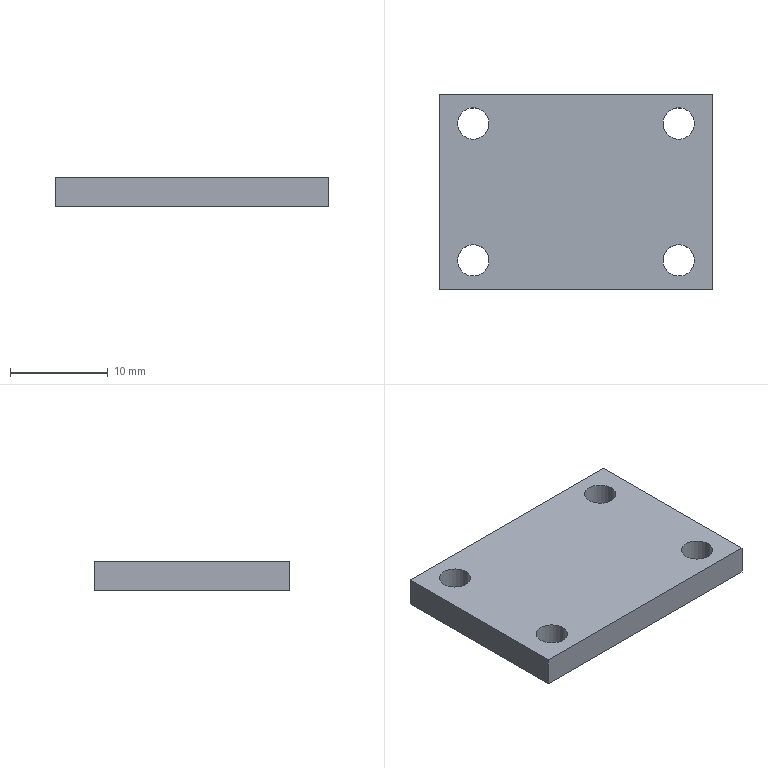Part | SolidWorks | features Extrusion 1 | 1 solid | 14 faces | box 28 x 20 x 3 mm | volume 1583 mm3 | cylinder 8 | plane 6 | commonest cylinder face diameters 3.2 x8
STEP:
#1=CARTESIAN_POINT('',(-12.1,-7.,1.5));
#2=VERTEX_POINT('',#1);
#3=CARTESIAN_POINT('',(-8.9,-7.,1.5));
#4=VERTEX_POINT('',#3);
#5=CARTESIAN_POINT('',(-10.5,-7.,1.5));
#6=DIRECTION('',(0.,0.,1.));
#7=DIRECTION('',(1.,0.,0.));
#8=AXIS2_PLACEMENT_3D('',#5,#6,#7);
#9=CIRCLE('',#8,1.6);
#10=EDGE_CURVE('',#2,#4,#9,.T.);
#11=ORIENTED_EDGE('',*,*,#10,.T.);
#12=CARTESIAN_POINT('',(-8.9,-7.,-1.5));
#13=VERTEX_POINT('',#12);
#14=CARTESIAN_POINT('',(-8.9,-7.,1.5));
#15=DIRECTION('',(0.,0.,-1.));
#16=VECTOR('',#15,1000.);
#17=LINE('',#14,#16);
#18=EDGE_CURVE('',#4,#13,#17,.T.);
#19=ORIENTED_EDGE('',*,*,#18,.T.);
#20=CARTESIAN_POINT('',(-12.1,-7.,-1.5));
#21=VERTEX_POINT('',#20);
#22=CARTESIAN_POINT('',(-10.5,-7.,-1.5));
#23=DIRECTION('',(0.,0.,1.));
#24=DIRECTION('',(1.,0.,0.));
#25=AXIS2_PLACEMENT_3D('',#22,#23,#24);
#26=CIRCLE('',#25,1.6);
#27=EDGE_CURVE('',#21,#13,#26,.T.);
#28=ORIENTED_EDGE('',*,*,#27,.F.);
#29=CARTESIAN_POINT('',(-12.1,-7.,1.5));
#30=DIRECTION('',(0.,0.,-1.));
#31=VECTOR('',#30,1000.);
#32=LINE('',#29,#31);
#33=EDGE_CURVE('',#2,#21,#32,.T.);
#34=ORIENTED_EDGE('',*,*,#33,.F.);
#35=EDGE_LOOP('',(#11,#19,#28,#34));
#36=FACE_OUTER_BOUND('',#35,.T.);
#37=CARTESIAN_POINT('',(-10.5,-7.,1.5));
#38=DIRECTION('',(0.,0.,-1.));
#39=DIRECTION('',(-1.,0.,0.));
#40=AXIS2_PLACEMENT_3D('',#37,#38,#39);
#41=CYLINDRICAL_SURFACE('',#40,1.6);
#42=ADVANCED_FACE('',(#36),#41,.F.);
#43=CARTESIAN_POINT('',(8.9,-7.,1.5));
#44=VERTEX_POINT('',#43);
#45=CARTESIAN_POINT('',(12.1,-7.,1.5));
#46=VERTEX_POINT('',#45);
#47=CARTESIAN_POINT('',(10.5,-7.,1.5));
#48=DIRECTION('',(0.,0.,1.));
#49=DIRECTION('',(-1.,0.,0.));
#50=AXIS2_PLACEMENT_3D('',#47,#48,#49);
#51=CIRCLE('',#50,1.6);
#52=EDGE_CURVE('',#44,#46,#51,.T.);
#53=ORIENTED_EDGE('',*,*,#52,.T.);
#54=CARTESIAN_POINT('',(12.1,-7.,-1.5));
#55=VERTEX_POINT('',#54);
#56=CARTESIAN_POINT('',(12.1,-7.,1.5));
#57=DIRECTION('',(0.,0.,-1.));
#58=VECTOR('',#57,1000.);
#59=LINE('',#56,#58);
#60=EDGE_CURVE('',#46,#55,#59,.T.);
#61=ORIENTED_EDGE('',*,*,#60,.T.);
#62=CARTESIAN_POINT('',(8.9,-7.,-1.5));
#63=VERTEX_POINT('',#62);
#64=CARTESIAN_POINT('',(10.5,-7.,-1.5));
#65=DIRECTION('',(0.,0.,1.));
#66=DIRECTION('',(-1.,0.,0.));
#67=AXIS2_PLACEMENT_3D('',#64,#65,#66);
#68=CIRCLE('',#67,1.6);
#69=EDGE_CURVE('',#63,#55,#68,.T.);
#70=ORIENTED_EDGE('',*,*,#69,.F.);
#71=CARTESIAN_POINT('',(8.9,-7.,1.5));
#72=DIRECTION('',(0.,0.,-1.));
#73=VECTOR('',#72,1000.);
#74=LINE('',#71,#73);
#75=EDGE_CURVE('',#44,#63,#74,.T.);
#76=ORIENTED_EDGE('',*,*,#75,.F.);
#77=EDGE_LOOP('',(#53,#61,#70,#76));
#78=FACE_OUTER_BOUND('',#77,.T.);
#79=CARTESIAN_POINT('',(10.5,-7.,1.5));
#80=DIRECTION('',(0.,0.,-1.));
#81=DIRECTION('',(-1.,0.,0.));
#82=AXIS2_PLACEMENT_3D('',#79,#80,#81);
#83=CYLINDRICAL_SURFACE('',#82,1.6);
#84=ADVANCED_FACE('',(#78),#83,.F.);
#85=CARTESIAN_POINT('',(-12.1,7.,1.5));
#86=VERTEX_POINT('',#85);
#87=CARTESIAN_POINT('',(-8.9,7.,1.5));
#88=VERTEX_POINT('',#87);
#89=CARTESIAN_POINT('',(-10.5,7.,1.5));
#90=DIRECTION('',(0.,0.,1.));
#91=DIRECTION('',(-1.,0.,0.));
#92=AXIS2_PLACEMENT_3D('',#89,#90,#91);
#93=CIRCLE('',#92,1.6);
#94=EDGE_CURVE('',#86,#88,#93,.T.);
#95=ORIENTED_EDGE('',*,*,#94,.T.);
#96=CARTESIAN_POINT('',(-8.9,7.,-1.5));
#97=VERTEX_POINT('',#96);
#98=CARTESIAN_POINT('',(-8.9,7.,1.5));
#99=DIRECTION('',(0.,0.,-1.));
#100=VECTOR('',#99,1000.);
#101=LINE('',#98,#100);
#102=EDGE_CURVE('',#88,#97,#101,.T.);
#103=ORIENTED_EDGE('',*,*,#102,.T.);
#104=CARTESIAN_POINT('',(-12.1,7.,-1.5));
#105=VERTEX_POINT('',#104);
#106=CARTESIAN_POINT('',(-10.5,7.,-1.5));
#107=DIRECTION('',(0.,0.,1.));
#108=DIRECTION('',(-1.,0.,0.));
#109=AXIS2_PLACEMENT_3D('',#106,#107,#108);
#110=CIRCLE('',#109,1.6);
#111=EDGE_CURVE('',#105,#97,#110,.T.);
#112=ORIENTED_EDGE('',*,*,#111,.F.);
#113=CARTESIAN_POINT('',(-12.1,7.,1.5));
#114=DIRECTION('',(0.,0.,-1.));
#115=VECTOR('',#114,1000.);
#116=LINE('',#113,#115);
#117=EDGE_CURVE('',#86,#105,#116,.T.);
#118=ORIENTED_EDGE('',*,*,#117,.F.);
#119=EDGE_LOOP('',(#95,#103,#112,#118));
#120=FACE_OUTER_BOUND('',#119,.T.);
#121=CARTESIAN_POINT('',(-10.5,7.,1.5));
#122=DIRECTION('',(0.,0.,-1.));
#123=DIRECTION('',(-1.,0.,0.));
#124=AXIS2_PLACEMENT_3D('',#121,#122,#123);
#125=CYLINDRICAL_SURFACE('',#124,1.6);
#126=ADVANCED_FACE('',(#120),#125,.F.);
#127=CARTESIAN_POINT('',(8.9,7.,1.5));
#128=VERTEX_POINT('',#127);
#129=CARTESIAN_POINT('',(12.1,7.,1.5));
#130=VERTEX_POINT('',#129);
#131=CARTESIAN_POINT('',(10.5,7.,1.5));
#132=DIRECTION('',(0.,0.,1.));
#133=DIRECTION('',(1.,0.,0.));
#134=AXIS2_PLACEMENT_3D('',#131,#132,#133);
#135=CIRCLE('',#134,1.6);
#136=EDGE_CURVE('',#128,#130,#135,.T.);
#137=ORIENTED_EDGE('',*,*,#136,.T.);
#138=CARTESIAN_POINT('',(12.1,7.,-1.5));
#139=VERTEX_POINT('',#138);
#140=CARTESIAN_POINT('',(12.1,7.,1.5));
#141=DIRECTION('',(0.,0.,-1.));
#142=VECTOR('',#141,1000.);
#143=LINE('',#140,#142);
#144=EDGE_CURVE('',#130,#139,#143,.T.);
#145=ORIENTED_EDGE('',*,*,#144,.T.);
#146=CARTESIAN_POINT('',(8.9,7.,-1.5));
#147=VERTEX_POINT('',#146);
#148=CARTESIAN_POINT('',(10.5,7.,-1.5));
#149=DIRECTION('',(0.,0.,1.));
#150=DIRECTION('',(1.,0.,0.));
#151=AXIS2_PLACEMENT_3D('',#148,#149,#150);
#152=CIRCLE('',#151,1.6);
#153=EDGE_CURVE('',#147,#139,#152,.T.);
#154=ORIENTED_EDGE('',*,*,#153,.F.);
#155=CARTESIAN_POINT('',(8.9,7.,1.5));
#156=DIRECTION('',(0.,0.,-1.));
#157=VECTOR('',#156,1000.);
#158=LINE('',#155,#157);
#159=EDGE_CURVE('',#128,#147,#158,.T.);
#160=ORIENTED_EDGE('',*,*,#159,.F.);
#161=EDGE_LOOP('',(#137,#145,#154,#160));
#162=FACE_OUTER_BOUND('',#161,.T.);
#163=CARTESIAN_POINT('',(10.5,7.,1.5));
#164=DIRECTION('',(0.,0.,-1.));
#165=DIRECTION('',(-1.,0.,0.));
#166=AXIS2_PLACEMENT_3D('',#163,#164,#165);
#167=CYLINDRICAL_SURFACE('',#166,1.6);
#168=ADVANCED_FACE('',(#162),#167,.F.);
#169=CARTESIAN_POINT('',(-14.,10.,1.5));
#170=VERTEX_POINT('',#169);
#171=CARTESIAN_POINT('',(-14.,-10.,1.5));
#172=VERTEX_POINT('',#171);
#173=CARTESIAN_POINT('',(-14.,10.,1.5));
#174=DIRECTION('',(0.,-1.,0.));
#175=VECTOR('',#174,1000.);
#176=LINE('',#173,#175);
#177=EDGE_CURVE('',#170,#172,#176,.T.);
#178=ORIENTED_EDGE('',*,*,#177,.T.);
#179=CARTESIAN_POINT('',(14.,-10.,1.5));
#180=VERTEX_POINT('',#179);
#181=CARTESIAN_POINT('',(14.,-10.,1.5));
#182=DIRECTION('',(1.,0.,0.));
#183=VECTOR('',#182,1000.);
#184=LINE('',#181,#183);
#185=EDGE_CURVE('',#172,#180,#184,.T.);
#186=ORIENTED_EDGE('',*,*,#185,.T.);
#187=CARTESIAN_POINT('',(14.,10.,1.5));
#188=VERTEX_POINT('',#187);
#189=CARTESIAN_POINT('',(14.,10.,1.5));
#190=DIRECTION('',(0.,1.,0.));
#191=VECTOR('',#190,1000.);
#192=LINE('',#189,#191);
#193=EDGE_CURVE('',#180,#188,#192,.T.);
#194=ORIENTED_EDGE('',*,*,#193,.T.);
#195=CARTESIAN_POINT('',(14.,10.,1.5));
#196=DIRECTION('',(-1.,0.,0.));
#197=VECTOR('',#196,1000.);
#198=LINE('',#195,#197);
#199=EDGE_CURVE('',#188,#170,#198,.T.);
#200=ORIENTED_EDGE('',*,*,#199,.T.);
#201=EDGE_LOOP('',(#178,#186,#194,#200));
#202=FACE_OUTER_BOUND('',#201,.T.);
#203=ORIENTED_EDGE('',*,*,#136,.F.);
#204=CARTESIAN_POINT('',(10.5,7.,1.5));
#205=DIRECTION('',(0.,0.,1.));
#206=DIRECTION('',(1.,0.,0.));
#207=AXIS2_PLACEMENT_3D('',#204,#205,#206);
#208=CIRCLE('',#207,1.6);
#209=EDGE_CURVE('',#130,#128,#208,.T.);
#210=ORIENTED_EDGE('',*,*,#209,.F.);
#211=EDGE_LOOP('',(#203,#210));
#212=FACE_BOUND('',#211,.T.);
#213=ORIENTED_EDGE('',*,*,#94,.F.);
#214=CARTESIAN_POINT('',(-10.5,7.,1.5));
#215=DIRECTION('',(0.,0.,1.));
#216=DIRECTION('',(-1.,0.,0.));
#217=AXIS2_PLACEMENT_3D('',#214,#215,#216);
#218=CIRCLE('',#217,1.6);
#219=EDGE_CURVE('',#88,#86,#218,.T.);
#220=ORIENTED_EDGE('',*,*,#219,.F.);
#221=EDGE_LOOP('',(#213,#220));
#222=FACE_BOUND('',#221,.T.);
#223=ORIENTED_EDGE('',*,*,#52,.F.);
#224=CARTESIAN_POINT('',(10.5,-7.,1.5));
#225=DIRECTION('',(0.,0.,1.));
#226=DIRECTION('',(-1.,0.,0.));
#227=AXIS2_PLACEMENT_3D('',#224,#225,#226);
#228=CIRCLE('',#227,1.6);
#229=EDGE_CURVE('',#46,#44,#228,.T.);
#230=ORIENTED_EDGE('',*,*,#229,.F.);
#231=EDGE_LOOP('',(#223,#230));
#232=FACE_BOUND('',#231,.T.);
#233=ORIENTED_EDGE('',*,*,#10,.F.);
#234=CARTESIAN_POINT('',(-10.5,-7.,1.5));
#235=DIRECTION('',(0.,0.,1.));
#236=DIRECTION('',(1.,0.,0.));
#237=AXIS2_PLACEMENT_3D('',#234,#235,#236);
#238=CIRCLE('',#237,1.6);
#239=EDGE_CURVE('',#4,#2,#238,.T.);
#240=ORIENTED_EDGE('',*,*,#239,.F.);
#241=EDGE_LOOP('',(#233,#240));
#242=FACE_BOUND('',#241,.T.);
#243=CARTESIAN_POINT('',(0.,0.,1.5));
#244=DIRECTION('',(0.,0.,-1.));
#245=DIRECTION('',(-1.,0.,0.));
#246=AXIS2_PLACEMENT_3D('',#243,#244,#245);
#247=PLANE('',#246);
#248=ADVANCED_FACE('',(#202,#212,#222,#232,#242),#247,.F.);
#249=ORIENTED_EDGE('',*,*,#69,.T.);
#250=CARTESIAN_POINT('',(10.5,-7.,-1.5));
#251=DIRECTION('',(0.,0.,1.));
#252=DIRECTION('',(-1.,0.,0.));
#253=AXIS2_PLACEMENT_3D('',#250,#251,#252);
#254=CIRCLE('',#253,1.6);
#255=EDGE_CURVE('',#55,#63,#254,.T.);
#256=ORIENTED_EDGE('',*,*,#255,.T.);
#257=EDGE_LOOP('',(#249,#256));
#258=FACE_BOUND('',#257,.T.);
#259=ORIENTED_EDGE('',*,*,#153,.T.);
#260=CARTESIAN_POINT('',(10.5,7.,-1.5));
#261=DIRECTION('',(0.,0.,1.));
#262=DIRECTION('',(1.,0.,0.));
#263=AXIS2_PLACEMENT_3D('',#260,#261,#262);
#264=CIRCLE('',#263,1.6);
#265=EDGE_CURVE('',#139,#147,#264,.T.);
#266=ORIENTED_EDGE('',*,*,#265,.T.);
#267=EDGE_LOOP('',(#259,#266));
#268=FACE_BOUND('',#267,.T.);
#269=CARTESIAN_POINT('',(-14.,10.,-1.5));
#270=VERTEX_POINT('',#269);
#271=CARTESIAN_POINT('',(-14.,-10.,-1.5));
#272=VERTEX_POINT('',#271);
#273=CARTESIAN_POINT('',(-14.,10.,-1.5));
#274=DIRECTION('',(0.,-1.,0.));
#275=VECTOR('',#274,1000.);
#276=LINE('',#273,#275);
#277=EDGE_CURVE('',#270,#272,#276,.T.);
#278=ORIENTED_EDGE('',*,*,#277,.F.);
#279=CARTESIAN_POINT('',(14.,10.,-1.5));
#280=VERTEX_POINT('',#279);
#281=CARTESIAN_POINT('',(14.,10.,-1.5));
#282=DIRECTION('',(-1.,0.,0.));
#283=VECTOR('',#282,1000.);
#284=LINE('',#281,#283);
#285=EDGE_CURVE('',#280,#270,#284,.T.);
#286=ORIENTED_EDGE('',*,*,#285,.F.);
#287=CARTESIAN_POINT('',(14.,-10.,-1.5));
#288=VERTEX_POINT('',#287);
#289=CARTESIAN_POINT('',(14.,10.,-1.5));
#290=DIRECTION('',(0.,1.,0.));
#291=VECTOR('',#290,1000.);
#292=LINE('',#289,#291);
#293=EDGE_CURVE('',#288,#280,#292,.T.);
#294=ORIENTED_EDGE('',*,*,#293,.F.);
#295=CARTESIAN_POINT('',(14.,-10.,-1.5));
#296=DIRECTION('',(1.,0.,0.));
#297=VECTOR('',#296,1000.);
#298=LINE('',#295,#297);
#299=EDGE_CURVE('',#272,#288,#298,.T.);
#300=ORIENTED_EDGE('',*,*,#299,.F.);
#301=EDGE_LOOP('',(#278,#286,#294,#300));
#302=FACE_OUTER_BOUND('',#301,.T.);
#303=ORIENTED_EDGE('',*,*,#111,.T.);
#304=CARTESIAN_POINT('',(-10.5,7.,-1.5));
#305=DIRECTION('',(0.,0.,1.));
#306=DIRECTION('',(-1.,0.,0.));
#307=AXIS2_PLACEMENT_3D('',#304,#305,#306);
#308=CIRCLE('',#307,1.6);
#309=EDGE_CURVE('',#97,#105,#308,.T.);
#310=ORIENTED_EDGE('',*,*,#309,.T.);
#311=EDGE_LOOP('',(#303,#310));
#312=FACE_BOUND('',#311,.T.);
#313=ORIENTED_EDGE('',*,*,#27,.T.);
#314=CARTESIAN_POINT('',(-10.5,-7.,-1.5));
#315=DIRECTION('',(0.,0.,1.));
#316=DIRECTION('',(1.,0.,0.));
#317=AXIS2_PLACEMENT_3D('',#314,#315,#316);
#318=CIRCLE('',#317,1.6);
#319=EDGE_CURVE('',#13,#21,#318,.T.);
#320=ORIENTED_EDGE('',*,*,#319,.T.);
#321=EDGE_LOOP('',(#313,#320));
#322=FACE_BOUND('',#321,.T.);
#323=CARTESIAN_POINT('',(0.,0.,-1.5));
#324=DIRECTION('',(0.,0.,-1.));
#325=DIRECTION('',(-1.,0.,0.));
#326=AXIS2_PLACEMENT_3D('',#323,#324,#325);
#327=PLANE('',#326);
#328=ADVANCED_FACE('',(#258,#268,#302,#312,#322),#327,.T.);
#329=ORIENTED_EDGE('',*,*,#277,.T.);
#330=CARTESIAN_POINT('',(-14.,-10.,1.5));
#331=DIRECTION('',(0.,0.,-1.));
#332=VECTOR('',#331,1000.);
#333=LINE('',#330,#332);
#334=EDGE_CURVE('',#172,#272,#333,.T.);
#335=ORIENTED_EDGE('',*,*,#334,.F.);
#336=ORIENTED_EDGE('',*,*,#177,.F.);
#337=CARTESIAN_POINT('',(-14.,10.,1.5));
#338=DIRECTION('',(0.,0.,-1.));
#339=VECTOR('',#338,1000.);
#340=LINE('',#337,#339);
#341=EDGE_CURVE('',#170,#270,#340,.T.);
#342=ORIENTED_EDGE('',*,*,#341,.T.);
#343=EDGE_LOOP('',(#329,#335,#336,#342));
#344=FACE_OUTER_BOUND('',#343,.T.);
#345=CARTESIAN_POINT('',(-14.,10.,1.5));
#346=DIRECTION('',(1.,0.,0.));
#347=DIRECTION('',(0.,1.,0.));
#348=AXIS2_PLACEMENT_3D('',#345,#346,#347);
#349=PLANE('',#348);
#350=ADVANCED_FACE('',(#344),#349,.F.);
#351=ORIENTED_EDGE('',*,*,#299,.T.);
#352=CARTESIAN_POINT('',(14.,-10.,1.5));
#353=DIRECTION('',(0.,0.,-1.));
#354=VECTOR('',#353,1000.);
#355=LINE('',#352,#354);
#356=EDGE_CURVE('',#180,#288,#355,.T.);
#357=ORIENTED_EDGE('',*,*,#356,.F.);
#358=ORIENTED_EDGE('',*,*,#185,.F.);
#359=ORIENTED_EDGE('',*,*,#334,.T.);
#360=EDGE_LOOP('',(#351,#357,#358,#359));
#361=FACE_OUTER_BOUND('',#360,.T.);
#362=CARTESIAN_POINT('',(14.,-10.,1.5));
#363=DIRECTION('',(0.,1.,0.));
#364=DIRECTION('',(-1.,0.,0.));
#365=AXIS2_PLACEMENT_3D('',#362,#363,#364);
#366=PLANE('',#365);
#367=ADVANCED_FACE('',(#361),#366,.F.);
#368=ORIENTED_EDGE('',*,*,#293,.T.);
#369=CARTESIAN_POINT('',(14.,10.,1.5));
#370=DIRECTION('',(0.,0.,-1.));
#371=VECTOR('',#370,1000.);
#372=LINE('',#369,#371);
#373=EDGE_CURVE('',#188,#280,#372,.T.);
#374=ORIENTED_EDGE('',*,*,#373,.F.);
#375=ORIENTED_EDGE('',*,*,#193,.F.);
#376=ORIENTED_EDGE('',*,*,#356,.T.);
#377=EDGE_LOOP('',(#368,#374,#375,#376));
#378=FACE_OUTER_BOUND('',#377,.T.);
#379=CARTESIAN_POINT('',(14.,10.,1.5));
#380=DIRECTION('',(-1.,0.,0.));
#381=DIRECTION('',(0.,0.,1.));
#382=AXIS2_PLACEMENT_3D('',#379,#380,#381);
#383=PLANE('',#382);
#384=ADVANCED_FACE('',(#378),#383,.F.);
#385=ORIENTED_EDGE('',*,*,#285,.T.);
#386=ORIENTED_EDGE('',*,*,#341,.F.);
#387=ORIENTED_EDGE('',*,*,#199,.F.);
#388=ORIENTED_EDGE('',*,*,#373,.T.);
#389=EDGE_LOOP('',(#385,#386,#387,#388));
#390=FACE_OUTER_BOUND('',#389,.T.);
#391=CARTESIAN_POINT('',(14.,10.,1.5));
#392=DIRECTION('',(0.,-1.,0.));
#393=DIRECTION('',(1.,0.,0.));
#394=AXIS2_PLACEMENT_3D('',#391,#392,#393);
#395=PLANE('',#394);
#396=ADVANCED_FACE('',(#390),#395,.F.);
#397=ORIENTED_EDGE('',*,*,#144,.F.);
#398=ORIENTED_EDGE('',*,*,#209,.T.);
#399=ORIENTED_EDGE('',*,*,#159,.T.);
#400=ORIENTED_EDGE('',*,*,#265,.F.);
#401=EDGE_LOOP('',(#397,#398,#399,#400));
#402=FACE_OUTER_BOUND('',#401,.T.);
#403=CARTESIAN_POINT('',(10.5,7.,1.5));
#404=DIRECTION('',(0.,0.,-1.));
#405=DIRECTION('',(-1.,0.,0.));
#406=AXIS2_PLACEMENT_3D('',#403,#404,#405);
#407=CYLINDRICAL_SURFACE('',#406,1.6);
#408=ADVANCED_FACE('',(#402),#407,.F.);
#409=ORIENTED_EDGE('',*,*,#102,.F.);
#410=ORIENTED_EDGE('',*,*,#219,.T.);
#411=ORIENTED_EDGE('',*,*,#117,.T.);
#412=ORIENTED_EDGE('',*,*,#309,.F.);
#413=EDGE_LOOP('',(#409,#410,#411,#412));
#414=FACE_OUTER_BOUND('',#413,.T.);
#415=CARTESIAN_POINT('',(-10.5,7.,1.5));
#416=DIRECTION('',(0.,0.,-1.));
#417=DIRECTION('',(-1.,0.,0.));
#418=AXIS2_PLACEMENT_3D('',#415,#416,#417);
#419=CYLINDRICAL_SURFACE('',#418,1.6);
#420=ADVANCED_FACE('',(#414),#419,.F.);
#421=ORIENTED_EDGE('',*,*,#60,.F.);
#422=ORIENTED_EDGE('',*,*,#229,.T.);
#423=ORIENTED_EDGE('',*,*,#75,.T.);
#424=ORIENTED_EDGE('',*,*,#255,.F.);
#425=EDGE_LOOP('',(#421,#422,#423,#424));
#426=FACE_OUTER_BOUND('',#425,.T.);
#427=CARTESIAN_POINT('',(10.5,-7.,1.5));
#428=DIRECTION('',(0.,0.,-1.));
#429=DIRECTION('',(-1.,0.,0.));
#430=AXIS2_PLACEMENT_3D('',#427,#428,#429);
#431=CYLINDRICAL_SURFACE('',#430,1.6);
#432=ADVANCED_FACE('',(#426),#431,.F.);
#433=ORIENTED_EDGE('',*,*,#18,.F.);
#434=ORIENTED_EDGE('',*,*,#239,.T.);
#435=ORIENTED_EDGE('',*,*,#33,.T.);
#436=ORIENTED_EDGE('',*,*,#319,.F.);
#437=EDGE_LOOP('',(#433,#434,#435,#436));
#438=FACE_OUTER_BOUND('',#437,.T.);
#439=CARTESIAN_POINT('',(-10.5,-7.,1.5));
#440=DIRECTION('',(0.,0.,-1.));
#441=DIRECTION('',(-1.,0.,0.));
#442=AXIS2_PLACEMENT_3D('',#439,#440,#441);
#443=CYLINDRICAL_SURFACE('',#442,1.6);
#444=ADVANCED_FACE('',(#438),#443,.F.);
#445=CLOSED_SHELL('',(#42,#84,#126,#168,#248,#328,#350,#367,#384,#396,#408,#420,#432,#444));
#446=MANIFOLD_SOLID_BREP('',#445);
#447=CARTESIAN_POINT('',(0.,0.,0.));
#448=DIRECTION('',(0.,0.,1.));
#449=DIRECTION('',(1.,0.,0.));
#450=AXIS2_PLACEMENT_3D('',#447,#448,#449);
#451=(LENGTH_UNIT()NAMED_UNIT(*)SI_UNIT(.MILLI.,.METRE.));
#452=UNCERTAINTY_MEASURE_WITH_UNIT(LENGTH_MEASURE(0.00001),#451,'','');
#453=(NAMED_UNIT(*)PLANE_ANGLE_UNIT()SI_UNIT($,.RADIAN.));
#454=(NAMED_UNIT(*)SI_UNIT($,.STERADIAN.)SOLID_ANGLE_UNIT());
#455=(GEOMETRIC_REPRESENTATION_CONTEXT(3)GLOBAL_UNCERTAINTY_ASSIGNED_CONTEXT((#452))GLOBAL_UNIT_ASSIGNED_CONTEXT((#451,#453,#454))REPRESENTATION_CONTEXT('',''));
#456=ADVANCED_BREP_SHAPE_REPRESENTATION('',(#446,#450),#455);